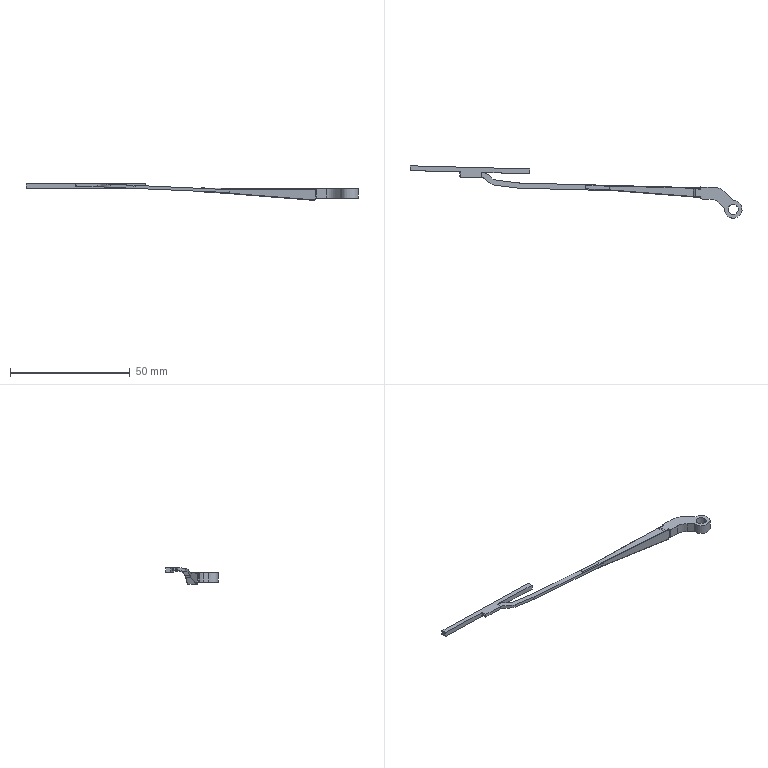Part | NX | features DATUM_CSYS 3, OFFSET_REGION 3, BREP 2, EXTRUDE 2, SKETCH 2, SCALE 1, UNITE 1 | 1 solid | 81 faces | box 138.697 x 21.869 x 6.967 mm | volume 1173 mm3 | plane 45 | cylinder 28 | spline 6 | torus 2 | commonest cylinder face diameters 0.4 x12 2 x6 0.8 x4 4.2 x1 7 x1 7.4 x1